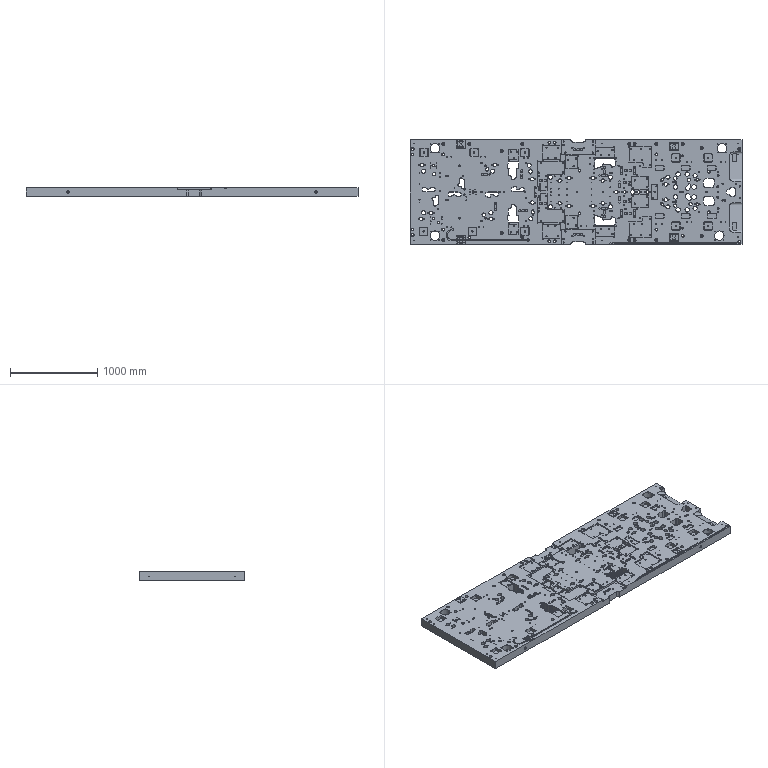Part | STEP file | lll_id5074_x_t | 1 solid | 2641 faces | box 3800 x 1200 x 100 mm | volume 402333507 mm3 | plane 1125 | cylinder 1001 | cone 414 | other 76 | spline 24 | torus 1 | commonest cylinder face diameters 14.506 x111 10 x76 8.506 x66 6.806 x60 10.506 x58 20 x46